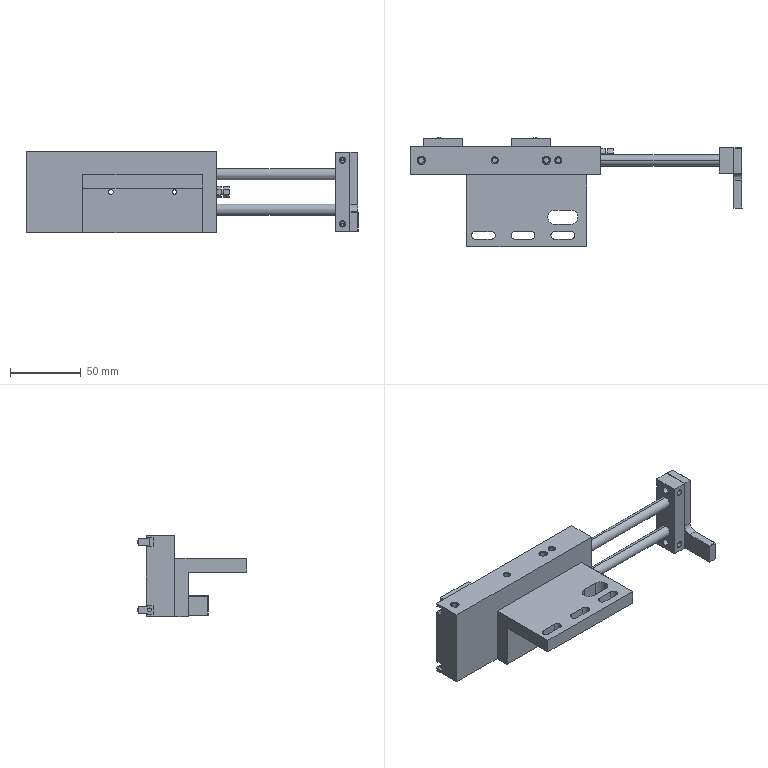Part | NX | 6 solids | 416 faces | box 235 x 77.196 x 58 mm | volume 229749 mm3 | plane 193 | cylinder 139 | cone 84 | commonest cylinder face diameters 4 x26 5 x18 3.4 x16 5.5 x13 2.5 x12 8 x12